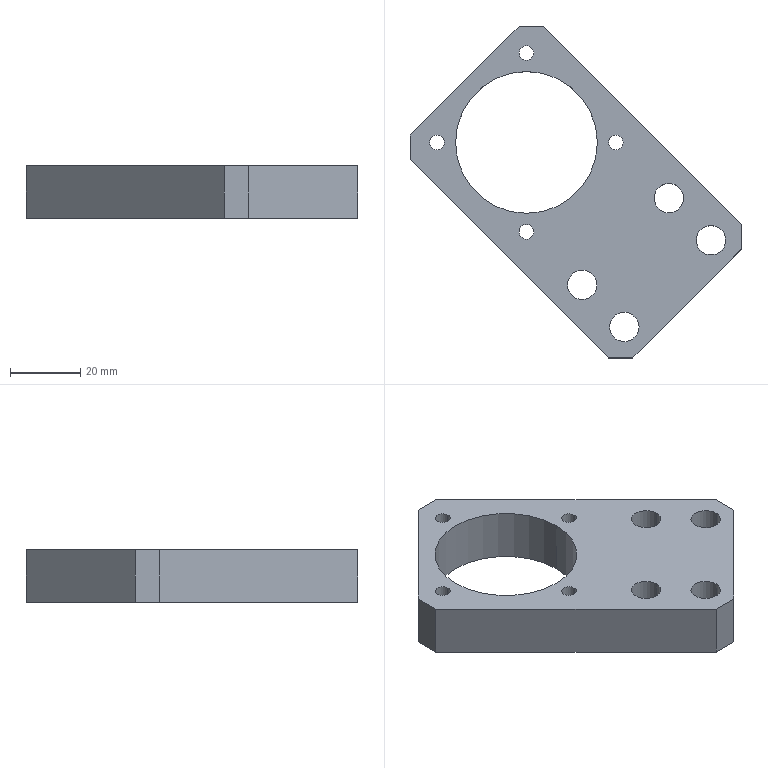Part | STEP file | 1 solid | 28 faces | box 94.752 x 94.752 x 15 mm | volume 48670 mm3 | cylinder 18 | plane 10 | commonest cylinder face diameters 4.2 x8 8.4 x8 40.5 x2